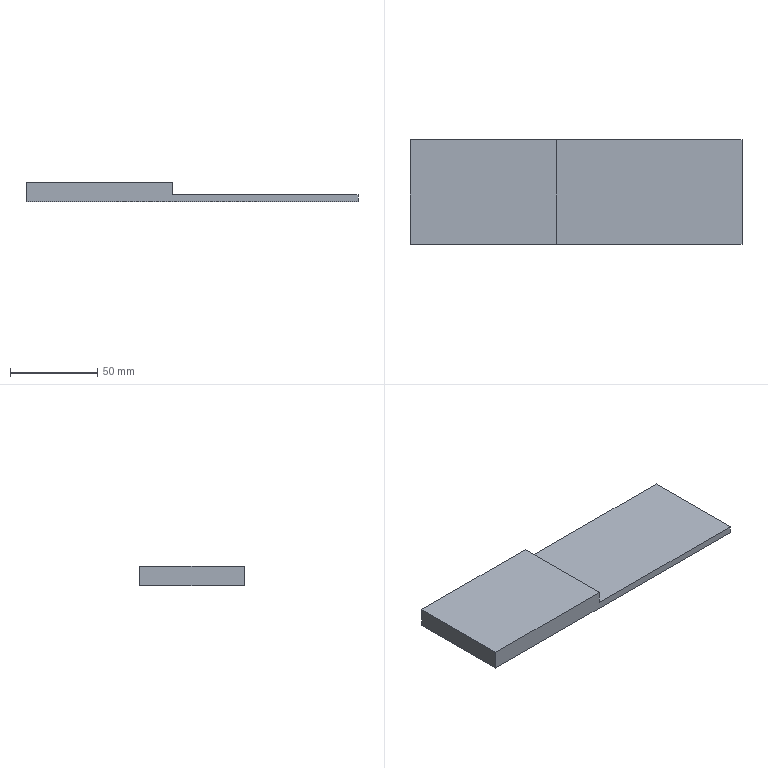Part | STEP file | Plate 1 | 1 solid | 8 faces | box 190 x 60 x 11 mm | volume 80880 mm3 | plane 8
STEP:
#1=CARTESIAN_POINT('',(-11.,-30.,4.));
#2=VERTEX_POINT('',#1);
#3=CARTESIAN_POINT('',(-11.,30.,4.));
#4=VERTEX_POINT('',#3);
#5=CARTESIAN_POINT('',(-11.,30.,4.));
#6=DIRECTION('',(0.,1.,0.));
#7=VECTOR('',#6,1000.);
#8=LINE('',#5,#7);
#9=EDGE_CURVE('',#2,#4,#8,.T.);
#10=ORIENTED_EDGE('',*,*,#9,.F.);
#11=CARTESIAN_POINT('',(95.,-30.,4.));
#12=VERTEX_POINT('',#11);
#13=CARTESIAN_POINT('',(-95.,-30.,4.));
#14=DIRECTION('',(1.,0.,0.));
#15=VECTOR('',#14,1000.);
#16=LINE('',#13,#15);
#17=EDGE_CURVE('',#2,#12,#16,.T.);
#18=ORIENTED_EDGE('',*,*,#17,.T.);
#19=CARTESIAN_POINT('',(95.,30.,4.));
#20=VERTEX_POINT('',#19);
#21=CARTESIAN_POINT('',(95.,-30.,4.));
#22=DIRECTION('',(0.,1.,0.));
#23=VECTOR('',#22,1000.);
#24=LINE('',#21,#23);
#25=EDGE_CURVE('',#12,#20,#24,.T.);
#26=ORIENTED_EDGE('',*,*,#25,.T.);
#27=CARTESIAN_POINT('',(-95.,30.,4.));
#28=DIRECTION('',(-1.,0.,0.));
#29=VECTOR('',#28,1000.);
#30=LINE('',#27,#29);
#31=EDGE_CURVE('',#20,#4,#30,.T.);
#32=ORIENTED_EDGE('',*,*,#31,.T.);
#33=EDGE_LOOP('',(#10,#18,#26,#32));
#34=FACE_OUTER_BOUND('',#33,.T.);
#35=CARTESIAN_POINT('',(0.,0.,4.));
#36=DIRECTION('',(0.,0.,-1.));
#37=DIRECTION('',(-1.,0.,0.));
#38=AXIS2_PLACEMENT_3D('',#35,#36,#37);
#39=PLANE('',#38);
#40=ADVANCED_FACE('',(#34),#39,.F.);
#41=CARTESIAN_POINT('',(95.,-30.,0.));
#42=VERTEX_POINT('',#41);
#43=CARTESIAN_POINT('',(95.,30.,0.));
#44=VERTEX_POINT('',#43);
#45=CARTESIAN_POINT('',(95.,-30.,0.));
#46=DIRECTION('',(0.,1.,0.));
#47=VECTOR('',#46,1000.);
#48=LINE('',#45,#47);
#49=EDGE_CURVE('',#42,#44,#48,.T.);
#50=ORIENTED_EDGE('',*,*,#49,.T.);
#51=CARTESIAN_POINT('',(95.,30.,4.));
#52=DIRECTION('',(0.,0.,-1.));
#53=VECTOR('',#52,1000.);
#54=LINE('',#51,#53);
#55=EDGE_CURVE('',#20,#44,#54,.T.);
#56=ORIENTED_EDGE('',*,*,#55,.F.);
#57=ORIENTED_EDGE('',*,*,#25,.F.);
#58=CARTESIAN_POINT('',(95.,-30.,4.));
#59=DIRECTION('',(0.,0.,-1.));
#60=VECTOR('',#59,1000.);
#61=LINE('',#58,#60);
#62=EDGE_CURVE('',#12,#42,#61,.T.);
#63=ORIENTED_EDGE('',*,*,#62,.T.);
#64=EDGE_LOOP('',(#50,#56,#57,#63));
#65=FACE_OUTER_BOUND('',#64,.T.);
#66=CARTESIAN_POINT('',(95.,-30.,4.));
#67=DIRECTION('',(-1.,0.,0.));
#68=DIRECTION('',(0.,0.,1.));
#69=AXIS2_PLACEMENT_3D('',#66,#67,#68);
#70=PLANE('',#69);
#71=ADVANCED_FACE('',(#65),#70,.F.);
#72=CARTESIAN_POINT('',(-95.,30.,0.));
#73=VERTEX_POINT('',#72);
#74=CARTESIAN_POINT('',(-95.,30.,0.));
#75=DIRECTION('',(-1.,0.,0.));
#76=VECTOR('',#75,1000.);
#77=LINE('',#74,#76);
#78=EDGE_CURVE('',#44,#73,#77,.T.);
#79=ORIENTED_EDGE('',*,*,#78,.T.);
#80=CARTESIAN_POINT('',(-95.,30.,11.));
#81=VERTEX_POINT('',#80);
#82=CARTESIAN_POINT('',(-95.,30.,4.));
#83=DIRECTION('',(0.,0.,-1.));
#84=VECTOR('',#83,1000.);
#85=LINE('',#82,#84);
#86=EDGE_CURVE('',#81,#73,#85,.T.);
#87=ORIENTED_EDGE('',*,*,#86,.F.);
#88=CARTESIAN_POINT('',(-11.,30.,11.));
#89=VERTEX_POINT('',#88);
#90=CARTESIAN_POINT('',(-95.,30.,11.));
#91=DIRECTION('',(-1.,0.,0.));
#92=VECTOR('',#91,1000.);
#93=LINE('',#90,#92);
#94=EDGE_CURVE('',#89,#81,#93,.T.);
#95=ORIENTED_EDGE('',*,*,#94,.F.);
#96=CARTESIAN_POINT('',(-11.,30.,11.));
#97=DIRECTION('',(0.,0.,-1.));
#98=VECTOR('',#97,1000.);
#99=LINE('',#96,#98);
#100=EDGE_CURVE('',#89,#4,#99,.T.);
#101=ORIENTED_EDGE('',*,*,#100,.T.);
#102=ORIENTED_EDGE('',*,*,#31,.F.);
#103=ORIENTED_EDGE('',*,*,#55,.T.);
#104=EDGE_LOOP('',(#79,#87,#95,#101,#102,#103));
#105=FACE_OUTER_BOUND('',#104,.T.);
#106=CARTESIAN_POINT('',(-95.,30.,4.));
#107=DIRECTION('',(0.,-1.,0.));
#108=DIRECTION('',(0.,0.,-1.));
#109=AXIS2_PLACEMENT_3D('',#106,#107,#108);
#110=PLANE('',#109);
#111=ADVANCED_FACE('',(#105),#110,.F.);
#112=CARTESIAN_POINT('',(-95.,-30.,0.));
#113=VERTEX_POINT('',#112);
#114=CARTESIAN_POINT('',(-95.,-30.,0.));
#115=DIRECTION('',(0.,-1.,0.));
#116=VECTOR('',#115,1000.);
#117=LINE('',#114,#116);
#118=EDGE_CURVE('',#73,#113,#117,.T.);
#119=ORIENTED_EDGE('',*,*,#118,.T.);
#120=CARTESIAN_POINT('',(-95.,-30.,11.));
#121=VERTEX_POINT('',#120);
#122=CARTESIAN_POINT('',(-95.,-30.,4.));
#123=DIRECTION('',(0.,0.,-1.));
#124=VECTOR('',#123,1000.);
#125=LINE('',#122,#124);
#126=EDGE_CURVE('',#121,#113,#125,.T.);
#127=ORIENTED_EDGE('',*,*,#126,.F.);
#128=CARTESIAN_POINT('',(-95.,30.,11.));
#129=DIRECTION('',(0.,-1.,0.));
#130=VECTOR('',#129,1000.);
#131=LINE('',#128,#130);
#132=EDGE_CURVE('',#81,#121,#131,.T.);
#133=ORIENTED_EDGE('',*,*,#132,.F.);
#134=ORIENTED_EDGE('',*,*,#86,.T.);
#135=EDGE_LOOP('',(#119,#127,#133,#134));
#136=FACE_OUTER_BOUND('',#135,.T.);
#137=CARTESIAN_POINT('',(-95.,-30.,4.));
#138=DIRECTION('',(1.,0.,0.));
#139=DIRECTION('',(0.,0.,-1.));
#140=AXIS2_PLACEMENT_3D('',#137,#138,#139);
#141=PLANE('',#140);
#142=ADVANCED_FACE('',(#136),#141,.F.);
#143=CARTESIAN_POINT('',(-95.,-30.,0.));
#144=DIRECTION('',(1.,0.,0.));
#145=VECTOR('',#144,1000.);
#146=LINE('',#143,#145);
#147=EDGE_CURVE('',#113,#42,#146,.T.);
#148=ORIENTED_EDGE('',*,*,#147,.T.);
#149=ORIENTED_EDGE('',*,*,#62,.F.);
#150=ORIENTED_EDGE('',*,*,#17,.F.);
#151=CARTESIAN_POINT('',(-11.,-30.,11.));
#152=VERTEX_POINT('',#151);
#153=CARTESIAN_POINT('',(-11.,-30.,11.));
#154=DIRECTION('',(0.,0.,-1.));
#155=VECTOR('',#154,1000.);
#156=LINE('',#153,#155);
#157=EDGE_CURVE('',#152,#2,#156,.T.);
#158=ORIENTED_EDGE('',*,*,#157,.F.);
#159=CARTESIAN_POINT('',(-95.,-30.,11.));
#160=DIRECTION('',(1.,0.,0.));
#161=VECTOR('',#160,1000.);
#162=LINE('',#159,#161);
#163=EDGE_CURVE('',#121,#152,#162,.T.);
#164=ORIENTED_EDGE('',*,*,#163,.F.);
#165=ORIENTED_EDGE('',*,*,#126,.T.);
#166=EDGE_LOOP('',(#148,#149,#150,#158,#164,#165));
#167=FACE_OUTER_BOUND('',#166,.T.);
#168=CARTESIAN_POINT('',(-95.,-30.,4.));
#169=DIRECTION('',(0.,1.,0.));
#170=DIRECTION('',(0.,0.,1.));
#171=AXIS2_PLACEMENT_3D('',#168,#169,#170);
#172=PLANE('',#171);
#173=ADVANCED_FACE('',(#167),#172,.F.);
#174=ORIENTED_EDGE('',*,*,#49,.F.);
#175=ORIENTED_EDGE('',*,*,#147,.F.);
#176=ORIENTED_EDGE('',*,*,#118,.F.);
#177=ORIENTED_EDGE('',*,*,#78,.F.);
#178=EDGE_LOOP('',(#174,#175,#176,#177));
#179=FACE_OUTER_BOUND('',#178,.T.);
#180=CARTESIAN_POINT('',(0.,0.,0.));
#181=DIRECTION('',(0.,0.,-1.));
#182=DIRECTION('',(-1.,0.,0.));
#183=AXIS2_PLACEMENT_3D('',#180,#181,#182);
#184=PLANE('',#183);
#185=ADVANCED_FACE('',(#179),#184,.T.);
#186=ORIENTED_EDGE('',*,*,#9,.T.);
#187=ORIENTED_EDGE('',*,*,#100,.F.);
#188=CARTESIAN_POINT('',(-11.,30.,11.));
#189=DIRECTION('',(0.,1.,0.));
#190=VECTOR('',#189,1000.);
#191=LINE('',#188,#190);
#192=EDGE_CURVE('',#152,#89,#191,.T.);
#193=ORIENTED_EDGE('',*,*,#192,.F.);
#194=ORIENTED_EDGE('',*,*,#157,.T.);
#195=EDGE_LOOP('',(#186,#187,#193,#194));
#196=FACE_OUTER_BOUND('',#195,.T.);
#197=CARTESIAN_POINT('',(-11.,30.,11.));
#198=DIRECTION('',(-1.,0.,0.));
#199=DIRECTION('',(0.,-1.,0.));
#200=AXIS2_PLACEMENT_3D('',#197,#198,#199);
#201=PLANE('',#200);
#202=ADVANCED_FACE('',(#196),#201,.F.);
#203=ORIENTED_EDGE('',*,*,#132,.T.);
#204=ORIENTED_EDGE('',*,*,#163,.T.);
#205=ORIENTED_EDGE('',*,*,#192,.T.);
#206=ORIENTED_EDGE('',*,*,#94,.T.);
#207=EDGE_LOOP('',(#203,#204,#205,#206));
#208=FACE_OUTER_BOUND('',#207,.T.);
#209=CARTESIAN_POINT('',(0.,0.,11.));
#210=DIRECTION('',(0.,0.,1.));
#211=DIRECTION('',(1.,0.,0.));
#212=AXIS2_PLACEMENT_3D('',#209,#210,#211);
#213=PLANE('',#212);
#214=ADVANCED_FACE('',(#208),#213,.T.);
#215=CLOSED_SHELL('',(#40,#71,#111,#142,#173,#185,#202,#214));
#216=MANIFOLD_SOLID_BREP('',#215);
#217=CARTESIAN_POINT('',(0.,0.,0.));
#218=DIRECTION('',(0.,0.,1.));
#219=DIRECTION('',(1.,0.,0.));
#220=AXIS2_PLACEMENT_3D('',#217,#218,#219);
#221=(LENGTH_UNIT()NAMED_UNIT(*)SI_UNIT(.MILLI.,.METRE.));
#222=UNCERTAINTY_MEASURE_WITH_UNIT(LENGTH_MEASURE(0.00001),#221,'','');
#223=(NAMED_UNIT(*)PLANE_ANGLE_UNIT()SI_UNIT($,.RADIAN.));
#224=(NAMED_UNIT(*)SI_UNIT($,.STERADIAN.)SOLID_ANGLE_UNIT());
#225=(GEOMETRIC_REPRESENTATION_CONTEXT(3)GLOBAL_UNCERTAINTY_ASSIGNED_CONTEXT((#222))GLOBAL_UNIT_ASSIGNED_CONTEXT((#221,#223,#224))REPRESENTATION_CONTEXT('',''));
#226=ADVANCED_BREP_SHAPE_REPRESENTATION('',(#216,#220),#225);